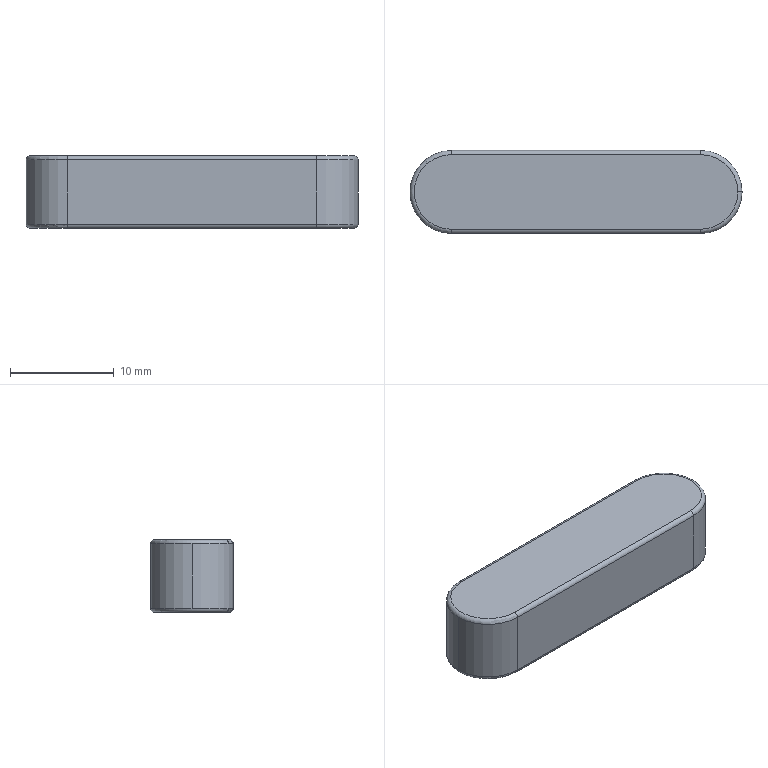Part | SolidWorks | features BaseBody 1 | 1 solid | 17 faces | box 32 x 8 x 7 mm | volume 1691 mm3 | cylinder 7 | torus 6 | plane 4 | commonest cylinder face diameters 0.8 x4 8 x3
STEP:
#1=CARTESIAN_POINT('',(15.6,0.,0.));
#2=VERTEX_POINT('',#1);
#3=CARTESIAN_POINT('',(16.,0.,0.4));
#4=VERTEX_POINT('',#3);
#5=CARTESIAN_POINT('',(15.6,0.,0.4));
#6=DIRECTION('',(0.,-1.,0.));
#7=DIRECTION('',(1.,0.,0.));
#8=AXIS2_PLACEMENT_3D('',#5,#6,#7);
#9=CIRCLE('',#8,0.4);
#10=EDGE_CURVE('',#2,#4,#9,.T.);
#11=ORIENTED_EDGE('',*,*,#10,.F.);
#12=CARTESIAN_POINT('',(12.,3.6,0.));
#13=VERTEX_POINT('',#12);
#14=CARTESIAN_POINT('',(12.,0.,0.));
#15=DIRECTION('',(0.,0.,-1.));
#16=DIRECTION('',(1.,0.,0.));
#17=AXIS2_PLACEMENT_3D('',#14,#15,#16);
#18=CIRCLE('',#17,3.6);
#19=EDGE_CURVE('',#13,#2,#18,.T.);
#20=ORIENTED_EDGE('',*,*,#19,.F.);
#21=CARTESIAN_POINT('',(12.,4.,0.4));
#22=VERTEX_POINT('',#21);
#23=CARTESIAN_POINT('',(12.,3.6,0.4));
#24=DIRECTION('',(1.,0.,0.));
#25=DIRECTION('',(0.,0.,-1.));
#26=AXIS2_PLACEMENT_3D('',#23,#24,#25);
#27=CIRCLE('',#26,0.4);
#28=EDGE_CURVE('',#13,#22,#27,.T.);
#29=ORIENTED_EDGE('',*,*,#28,.T.);
#30=CARTESIAN_POINT('',(12.,0.,0.4));
#31=DIRECTION('',(0.,0.,1.));
#32=DIRECTION('',(1.,0.,0.));
#33=AXIS2_PLACEMENT_3D('',#30,#31,#32);
#34=CIRCLE('',#33,4.);
#35=EDGE_CURVE('',#4,#22,#34,.T.);
#36=ORIENTED_EDGE('',*,*,#35,.F.);
#37=EDGE_LOOP('',(#11,#20,#29,#36));
#38=FACE_OUTER_BOUND('',#37,.T.);
#39=CARTESIAN_POINT('',(12.,0.,0.4));
#40=DIRECTION('',(0.,0.,1.));
#41=DIRECTION('',(1.,0.,0.));
#42=AXIS2_PLACEMENT_3D('',#39,#40,#41);
#43=TOROIDAL_SURFACE('',#42,3.6,0.4);
#44=ADVANCED_FACE('',(#38),#43,.T.);
#45=CARTESIAN_POINT('',(-12.,3.6,0.));
#46=VERTEX_POINT('',#45);
#47=CARTESIAN_POINT('',(-12.,4.,0.4));
#48=VERTEX_POINT('',#47);
#49=CARTESIAN_POINT('',(-12.,3.6,0.4));
#50=DIRECTION('',(1.,0.,0.));
#51=DIRECTION('',(0.,0.,-1.));
#52=AXIS2_PLACEMENT_3D('',#49,#50,#51);
#53=CIRCLE('',#52,0.4);
#54=EDGE_CURVE('',#46,#48,#53,.T.);
#55=ORIENTED_EDGE('',*,*,#54,.T.);
#56=CARTESIAN_POINT('',(-12.,4.,0.4));
#57=DIRECTION('',(-1.,0.,0.));
#58=VECTOR('',#57,1000.);
#59=LINE('',#56,#58);
#60=EDGE_CURVE('',#22,#48,#59,.T.);
#61=ORIENTED_EDGE('',*,*,#60,.F.);
#62=ORIENTED_EDGE('',*,*,#28,.F.);
#63=CARTESIAN_POINT('',(-12.,3.6,0.));
#64=DIRECTION('',(1.,0.,0.));
#65=VECTOR('',#64,1000.);
#66=LINE('',#63,#65);
#67=EDGE_CURVE('',#46,#13,#66,.T.);
#68=ORIENTED_EDGE('',*,*,#67,.F.);
#69=EDGE_LOOP('',(#55,#61,#62,#68));
#70=FACE_OUTER_BOUND('',#69,.T.);
#71=CARTESIAN_POINT('',(-12.,3.6,0.4));
#72=DIRECTION('',(-1.,0.,0.));
#73=DIRECTION('',(0.,-1.,0.));
#74=AXIS2_PLACEMENT_3D('',#71,#72,#73);
#75=CYLINDRICAL_SURFACE('',#74,0.4);
#76=ADVANCED_FACE('',(#70),#75,.T.);
#77=CARTESIAN_POINT('',(-12.,-4.,0.4));
#78=VERTEX_POINT('',#77);
#79=CARTESIAN_POINT('',(-12.,-3.6,0.));
#80=VERTEX_POINT('',#79);
#81=CARTESIAN_POINT('',(-12.,-3.6,0.4));
#82=DIRECTION('',(1.,0.,0.));
#83=DIRECTION('',(0.,0.,-1.));
#84=AXIS2_PLACEMENT_3D('',#81,#82,#83);
#85=CIRCLE('',#84,0.4);
#86=EDGE_CURVE('',#78,#80,#85,.T.);
#87=ORIENTED_EDGE('',*,*,#86,.T.);
#88=CARTESIAN_POINT('',(12.,-3.6,0.));
#89=VERTEX_POINT('',#88);
#90=CARTESIAN_POINT('',(-12.,-3.6,0.));
#91=DIRECTION('',(-1.,0.,0.));
#92=VECTOR('',#91,1000.);
#93=LINE('',#90,#92);
#94=EDGE_CURVE('',#89,#80,#93,.T.);
#95=ORIENTED_EDGE('',*,*,#94,.F.);
#96=CARTESIAN_POINT('',(12.,-4.,0.4));
#97=VERTEX_POINT('',#96);
#98=CARTESIAN_POINT('',(12.,-3.6,0.4));
#99=DIRECTION('',(1.,0.,0.));
#100=DIRECTION('',(0.,0.,-1.));
#101=AXIS2_PLACEMENT_3D('',#98,#99,#100);
#102=CIRCLE('',#101,0.4);
#103=EDGE_CURVE('',#97,#89,#102,.T.);
#104=ORIENTED_EDGE('',*,*,#103,.F.);
#105=CARTESIAN_POINT('',(-12.,-4.,0.4));
#106=DIRECTION('',(1.,0.,0.));
#107=VECTOR('',#106,1000.);
#108=LINE('',#105,#107);
#109=EDGE_CURVE('',#78,#97,#108,.T.);
#110=ORIENTED_EDGE('',*,*,#109,.F.);
#111=EDGE_LOOP('',(#87,#95,#104,#110));
#112=FACE_OUTER_BOUND('',#111,.T.);
#113=CARTESIAN_POINT('',(-12.,-3.6,0.4));
#114=DIRECTION('',(1.,0.,0.));
#115=DIRECTION('',(0.,1.,0.));
#116=AXIS2_PLACEMENT_3D('',#113,#114,#115);
#117=CYLINDRICAL_SURFACE('',#116,0.4);
#118=ADVANCED_FACE('',(#112),#117,.T.);
#119=ORIENTED_EDGE('',*,*,#54,.F.);
#120=CARTESIAN_POINT('',(-12.,0.,0.));
#121=DIRECTION('',(0.,0.,-1.));
#122=DIRECTION('',(1.,0.,0.));
#123=AXIS2_PLACEMENT_3D('',#120,#121,#122);
#124=CIRCLE('',#123,3.6);
#125=EDGE_CURVE('',#80,#46,#124,.T.);
#126=ORIENTED_EDGE('',*,*,#125,.F.);
#127=ORIENTED_EDGE('',*,*,#86,.F.);
#128=CARTESIAN_POINT('',(-16.,0.,0.4));
#129=VERTEX_POINT('',#128);
#130=CARTESIAN_POINT('',(-12.,0.,0.4));
#131=DIRECTION('',(0.,0.,1.));
#132=DIRECTION('',(1.,0.,0.));
#133=AXIS2_PLACEMENT_3D('',#130,#131,#132);
#134=CIRCLE('',#133,4.);
#135=EDGE_CURVE('',#129,#78,#134,.T.);
#136=ORIENTED_EDGE('',*,*,#135,.F.);
#137=CARTESIAN_POINT('',(-12.,0.,0.4));
#138=DIRECTION('',(0.,0.,1.));
#139=DIRECTION('',(1.,0.,0.));
#140=AXIS2_PLACEMENT_3D('',#137,#138,#139);
#141=CIRCLE('',#140,4.);
#142=EDGE_CURVE('',#48,#129,#141,.T.);
#143=ORIENTED_EDGE('',*,*,#142,.F.);
#144=EDGE_LOOP('',(#119,#126,#127,#136,#143));
#145=FACE_OUTER_BOUND('',#144,.T.);
#146=CARTESIAN_POINT('',(-12.,0.,0.4));
#147=DIRECTION('',(0.,0.,1.));
#148=DIRECTION('',(1.,0.,0.));
#149=AXIS2_PLACEMENT_3D('',#146,#147,#148);
#150=TOROIDAL_SURFACE('',#149,3.6,0.4);
#151=ADVANCED_FACE('',(#145),#150,.T.);
#152=CARTESIAN_POINT('',(16.,0.,6.6));
#153=VERTEX_POINT('',#152);
#154=CARTESIAN_POINT('',(15.6,0.,7.));
#155=VERTEX_POINT('',#154);
#156=CARTESIAN_POINT('',(15.6,0.,6.6));
#157=DIRECTION('',(0.,-1.,0.));
#158=DIRECTION('',(1.,0.,0.));
#159=AXIS2_PLACEMENT_3D('',#156,#157,#158);
#160=CIRCLE('',#159,0.4);
#161=EDGE_CURVE('',#153,#155,#160,.T.);
#162=ORIENTED_EDGE('',*,*,#161,.F.);
#163=CARTESIAN_POINT('',(12.,4.,6.6));
#164=VERTEX_POINT('',#163);
#165=CARTESIAN_POINT('',(12.,0.,6.6));
#166=DIRECTION('',(0.,0.,-1.));
#167=DIRECTION('',(1.,0.,0.));
#168=AXIS2_PLACEMENT_3D('',#165,#166,#167);
#169=CIRCLE('',#168,4.);
#170=EDGE_CURVE('',#164,#153,#169,.T.);
#171=ORIENTED_EDGE('',*,*,#170,.F.);
#172=CARTESIAN_POINT('',(12.,3.6,7.));
#173=VERTEX_POINT('',#172);
#174=CARTESIAN_POINT('',(12.,3.6,6.6));
#175=DIRECTION('',(1.,0.,0.));
#176=DIRECTION('',(0.,0.,-1.));
#177=AXIS2_PLACEMENT_3D('',#174,#175,#176);
#178=CIRCLE('',#177,0.4);
#179=EDGE_CURVE('',#164,#173,#178,.T.);
#180=ORIENTED_EDGE('',*,*,#179,.T.);
#181=CARTESIAN_POINT('',(12.,0.,7.));
#182=DIRECTION('',(0.,0.,1.));
#183=DIRECTION('',(1.,0.,0.));
#184=AXIS2_PLACEMENT_3D('',#181,#182,#183);
#185=CIRCLE('',#184,3.6);
#186=EDGE_CURVE('',#155,#173,#185,.T.);
#187=ORIENTED_EDGE('',*,*,#186,.F.);
#188=EDGE_LOOP('',(#162,#171,#180,#187));
#189=FACE_OUTER_BOUND('',#188,.T.);
#190=CARTESIAN_POINT('',(12.,0.,6.6));
#191=DIRECTION('',(0.,0.,1.));
#192=DIRECTION('',(1.,0.,0.));
#193=AXIS2_PLACEMENT_3D('',#190,#191,#192);
#194=TOROIDAL_SURFACE('',#193,3.6,0.4);
#195=ADVANCED_FACE('',(#189),#194,.T.);
#196=CARTESIAN_POINT('',(-12.,4.,6.6));
#197=VERTEX_POINT('',#196);
#198=CARTESIAN_POINT('',(-12.,3.6,7.));
#199=VERTEX_POINT('',#198);
#200=CARTESIAN_POINT('',(-12.,3.6,6.6));
#201=DIRECTION('',(1.,0.,0.));
#202=DIRECTION('',(0.,0.,-1.));
#203=AXIS2_PLACEMENT_3D('',#200,#201,#202);
#204=CIRCLE('',#203,0.4);
#205=EDGE_CURVE('',#197,#199,#204,.T.);
#206=ORIENTED_EDGE('',*,*,#205,.T.);
#207=CARTESIAN_POINT('',(-12.,3.6,7.));
#208=DIRECTION('',(-1.,0.,0.));
#209=VECTOR('',#208,1000.);
#210=LINE('',#207,#209);
#211=EDGE_CURVE('',#173,#199,#210,.T.);
#212=ORIENTED_EDGE('',*,*,#211,.F.);
#213=ORIENTED_EDGE('',*,*,#179,.F.);
#214=CARTESIAN_POINT('',(12.,4.,6.6));
#215=DIRECTION('',(1.,0.,0.));
#216=VECTOR('',#215,1000.);
#217=LINE('',#214,#216);
#218=EDGE_CURVE('',#197,#164,#217,.T.);
#219=ORIENTED_EDGE('',*,*,#218,.F.);
#220=EDGE_LOOP('',(#206,#212,#213,#219));
#221=FACE_OUTER_BOUND('',#220,.T.);
#222=CARTESIAN_POINT('',(-12.,3.6,6.6));
#223=DIRECTION('',(1.,0.,0.));
#224=DIRECTION('',(0.,1.,0.));
#225=AXIS2_PLACEMENT_3D('',#222,#223,#224);
#226=CYLINDRICAL_SURFACE('',#225,0.4);
#227=ADVANCED_FACE('',(#221),#226,.T.);
#228=CARTESIAN_POINT('',(-12.,-3.6,7.));
#229=VERTEX_POINT('',#228);
#230=CARTESIAN_POINT('',(-12.,-4.,6.6));
#231=VERTEX_POINT('',#230);
#232=CARTESIAN_POINT('',(-12.,-3.6,6.6));
#233=DIRECTION('',(1.,0.,0.));
#234=DIRECTION('',(0.,0.,-1.));
#235=AXIS2_PLACEMENT_3D('',#232,#233,#234);
#236=CIRCLE('',#235,0.4);
#237=EDGE_CURVE('',#229,#231,#236,.T.);
#238=ORIENTED_EDGE('',*,*,#237,.T.);
#239=CARTESIAN_POINT('',(12.,-4.,6.6));
#240=VERTEX_POINT('',#239);
#241=CARTESIAN_POINT('',(-12.,-4.,6.6));
#242=DIRECTION('',(-1.,0.,0.));
#243=VECTOR('',#242,1000.);
#244=LINE('',#241,#243);
#245=EDGE_CURVE('',#240,#231,#244,.T.);
#246=ORIENTED_EDGE('',*,*,#245,.F.);
#247=CARTESIAN_POINT('',(12.,-3.6,7.));
#248=VERTEX_POINT('',#247);
#249=CARTESIAN_POINT('',(12.,-3.6,6.6));
#250=DIRECTION('',(1.,0.,0.));
#251=DIRECTION('',(0.,0.,-1.));
#252=AXIS2_PLACEMENT_3D('',#249,#250,#251);
#253=CIRCLE('',#252,0.4);
#254=EDGE_CURVE('',#248,#240,#253,.T.);
#255=ORIENTED_EDGE('',*,*,#254,.F.);
#256=CARTESIAN_POINT('',(12.,-3.6,7.));
#257=DIRECTION('',(1.,0.,0.));
#258=VECTOR('',#257,1000.);
#259=LINE('',#256,#258);
#260=EDGE_CURVE('',#229,#248,#259,.T.);
#261=ORIENTED_EDGE('',*,*,#260,.F.);
#262=EDGE_LOOP('',(#238,#246,#255,#261));
#263=FACE_OUTER_BOUND('',#262,.T.);
#264=CARTESIAN_POINT('',(-12.,-3.6,6.6));
#265=DIRECTION('',(-1.,0.,0.));
#266=DIRECTION('',(0.,-1.,0.));
#267=AXIS2_PLACEMENT_3D('',#264,#265,#266);
#268=CYLINDRICAL_SURFACE('',#267,0.4);
#269=ADVANCED_FACE('',(#263),#268,.T.);
#270=ORIENTED_EDGE('',*,*,#205,.F.);
#271=CARTESIAN_POINT('',(-16.,0.,6.6));
#272=VERTEX_POINT('',#271);
#273=CARTESIAN_POINT('',(-12.,0.,6.6));
#274=DIRECTION('',(0.,0.,-1.));
#275=DIRECTION('',(1.,0.,0.));
#276=AXIS2_PLACEMENT_3D('',#273,#274,#275);
#277=CIRCLE('',#276,4.);
#278=EDGE_CURVE('',#272,#197,#277,.T.);
#279=ORIENTED_EDGE('',*,*,#278,.F.);
#280=CARTESIAN_POINT('',(-12.,0.,6.6));
#281=DIRECTION('',(0.,0.,-1.));
#282=DIRECTION('',(1.,0.,0.));
#283=AXIS2_PLACEMENT_3D('',#280,#281,#282);
#284=CIRCLE('',#283,4.);
#285=EDGE_CURVE('',#231,#272,#284,.T.);
#286=ORIENTED_EDGE('',*,*,#285,.F.);
#287=ORIENTED_EDGE('',*,*,#237,.F.);
#288=CARTESIAN_POINT('',(-12.,0.,7.));
#289=DIRECTION('',(0.,0.,1.));
#290=DIRECTION('',(1.,0.,0.));
#291=AXIS2_PLACEMENT_3D('',#288,#289,#290);
#292=CIRCLE('',#291,3.6);
#293=EDGE_CURVE('',#199,#229,#292,.T.);
#294=ORIENTED_EDGE('',*,*,#293,.F.);
#295=EDGE_LOOP('',(#270,#279,#286,#287,#294));
#296=FACE_OUTER_BOUND('',#295,.T.);
#297=CARTESIAN_POINT('',(-12.,0.,6.6));
#298=DIRECTION('',(0.,0.,1.));
#299=DIRECTION('',(1.,0.,0.));
#300=AXIS2_PLACEMENT_3D('',#297,#298,#299);
#301=TOROIDAL_SURFACE('',#300,3.6,0.4);
#302=ADVANCED_FACE('',(#296),#301,.T.);
#303=ORIENTED_EDGE('',*,*,#67,.T.);
#304=ORIENTED_EDGE('',*,*,#19,.T.);
#305=CARTESIAN_POINT('',(12.,0.,0.));
#306=DIRECTION('',(0.,0.,-1.));
#307=DIRECTION('',(1.,0.,0.));
#308=AXIS2_PLACEMENT_3D('',#305,#306,#307);
#309=CIRCLE('',#308,3.6);
#310=EDGE_CURVE('',#2,#89,#309,.T.);
#311=ORIENTED_EDGE('',*,*,#310,.T.);
#312=ORIENTED_EDGE('',*,*,#94,.T.);
#313=ORIENTED_EDGE('',*,*,#125,.T.);
#314=EDGE_LOOP('',(#303,#304,#311,#312,#313));
#315=FACE_OUTER_BOUND('',#314,.T.);
#316=CARTESIAN_POINT('',(-12.,0.,0.));
#317=DIRECTION('',(0.,0.,1.));
#318=DIRECTION('',(0.,-1.,0.));
#319=AXIS2_PLACEMENT_3D('',#316,#317,#318);
#320=PLANE('',#319);
#321=ADVANCED_FACE('',(#315),#320,.F.);
#322=ORIENTED_EDGE('',*,*,#260,.T.);
#323=CARTESIAN_POINT('',(12.,0.,7.));
#324=DIRECTION('',(0.,0.,1.));
#325=DIRECTION('',(1.,0.,0.));
#326=AXIS2_PLACEMENT_3D('',#323,#324,#325);
#327=CIRCLE('',#326,3.6);
#328=EDGE_CURVE('',#248,#155,#327,.T.);
#329=ORIENTED_EDGE('',*,*,#328,.T.);
#330=ORIENTED_EDGE('',*,*,#186,.T.);
#331=ORIENTED_EDGE('',*,*,#211,.T.);
#332=ORIENTED_EDGE('',*,*,#293,.T.);
#333=EDGE_LOOP('',(#322,#329,#330,#331,#332));
#334=FACE_OUTER_BOUND('',#333,.T.);
#335=CARTESIAN_POINT('',(-12.,0.,7.));
#336=DIRECTION('',(0.,0.,1.));
#337=DIRECTION('',(0.,-1.,0.));
#338=AXIS2_PLACEMENT_3D('',#335,#336,#337);
#339=PLANE('',#338);
#340=ADVANCED_FACE('',(#334),#339,.T.);
#341=CARTESIAN_POINT('',(-12.,4.,7.));
#342=DIRECTION('',(0.,0.,-1.));
#343=VECTOR('',#342,1000.);
#344=LINE('',#341,#343);
#345=EDGE_CURVE('',#197,#48,#344,.T.);
#346=ORIENTED_EDGE('',*,*,#345,.F.);
#347=ORIENTED_EDGE('',*,*,#218,.T.);
#348=CARTESIAN_POINT('',(12.,4.,7.));
#349=DIRECTION('',(0.,0.,-1.));
#350=VECTOR('',#349,1000.);
#351=LINE('',#348,#350);
#352=EDGE_CURVE('',#164,#22,#351,.T.);
#353=ORIENTED_EDGE('',*,*,#352,.T.);
#354=ORIENTED_EDGE('',*,*,#60,.T.);
#355=EDGE_LOOP('',(#346,#347,#353,#354));
#356=FACE_OUTER_BOUND('',#355,.T.);
#357=CARTESIAN_POINT('',(-12.,4.,7.));
#358=DIRECTION('',(0.,-1.,0.));
#359=DIRECTION('',(0.,0.,-1.));
#360=AXIS2_PLACEMENT_3D('',#357,#358,#359);
#361=PLANE('',#360);
#362=ADVANCED_FACE('',(#356),#361,.F.);
#363=ORIENTED_EDGE('',*,*,#352,.F.);
#364=ORIENTED_EDGE('',*,*,#170,.T.);
#365=CARTESIAN_POINT('',(12.,0.,6.6));
#366=DIRECTION('',(0.,0.,-1.));
#367=DIRECTION('',(1.,0.,0.));
#368=AXIS2_PLACEMENT_3D('',#365,#366,#367);
#369=CIRCLE('',#368,4.);
#370=EDGE_CURVE('',#153,#240,#369,.T.);
#371=ORIENTED_EDGE('',*,*,#370,.T.);
#372=CARTESIAN_POINT('',(12.,-4.,7.));
#373=DIRECTION('',(0.,0.,-1.));
#374=VECTOR('',#373,1000.);
#375=LINE('',#372,#374);
#376=EDGE_CURVE('',#240,#97,#375,.T.);
#377=ORIENTED_EDGE('',*,*,#376,.T.);
#378=CARTESIAN_POINT('',(12.,0.,0.4));
#379=DIRECTION('',(0.,0.,1.));
#380=DIRECTION('',(1.,0.,0.));
#381=AXIS2_PLACEMENT_3D('',#378,#379,#380);
#382=CIRCLE('',#381,4.);
#383=EDGE_CURVE('',#97,#4,#382,.T.);
#384=ORIENTED_EDGE('',*,*,#383,.T.);
#385=ORIENTED_EDGE('',*,*,#35,.T.);
#386=EDGE_LOOP('',(#363,#364,#371,#377,#384,#385));
#387=FACE_OUTER_BOUND('',#386,.T.);
#388=CARTESIAN_POINT('',(12.,0.,7.));
#389=DIRECTION('',(0.,0.,-1.));
#390=DIRECTION('',(-1.,0.,0.));
#391=AXIS2_PLACEMENT_3D('',#388,#389,#390);
#392=CYLINDRICAL_SURFACE('',#391,4.);
#393=ADVANCED_FACE('',(#387),#392,.T.);
#394=ORIENTED_EDGE('',*,*,#376,.F.);
#395=ORIENTED_EDGE('',*,*,#245,.T.);
#396=CARTESIAN_POINT('',(-12.,-4.,7.));
#397=DIRECTION('',(0.,0.,-1.));
#398=VECTOR('',#397,1000.);
#399=LINE('',#396,#398);
#400=EDGE_CURVE('',#231,#78,#399,.T.);
#401=ORIENTED_EDGE('',*,*,#400,.T.);
#402=ORIENTED_EDGE('',*,*,#109,.T.);
#403=EDGE_LOOP('',(#394,#395,#401,#402));
#404=FACE_OUTER_BOUND('',#403,.T.);
#405=CARTESIAN_POINT('',(-12.,-4.,7.));
#406=DIRECTION('',(0.,1.,0.));
#407=DIRECTION('',(1.,0.,0.));
#408=AXIS2_PLACEMENT_3D('',#405,#406,#407);
#409=PLANE('',#408);
#410=ADVANCED_FACE('',(#404),#409,.F.);
#411=CARTESIAN_POINT('',(-16.,0.,7.));
#412=DIRECTION('',(0.,0.,-1.));
#413=VECTOR('',#412,1000.);
#414=LINE('',#411,#413);
#415=EDGE_CURVE('',#272,#129,#414,.T.);
#416=ORIENTED_EDGE('',*,*,#415,.F.);
#417=ORIENTED_EDGE('',*,*,#278,.T.);
#418=ORIENTED_EDGE('',*,*,#345,.T.);
#419=ORIENTED_EDGE('',*,*,#142,.T.);
#420=EDGE_LOOP('',(#416,#417,#418,#419));
#421=FACE_OUTER_BOUND('',#420,.T.);
#422=CARTESIAN_POINT('',(-12.,0.,7.));
#423=DIRECTION('',(0.,0.,-1.));
#424=DIRECTION('',(-1.,0.,0.));
#425=AXIS2_PLACEMENT_3D('',#422,#423,#424);
#426=CYLINDRICAL_SURFACE('',#425,4.);
#427=ADVANCED_FACE('',(#421),#426,.T.);
#428=ORIENTED_EDGE('',*,*,#285,.T.);
#429=ORIENTED_EDGE('',*,*,#415,.T.);
#430=ORIENTED_EDGE('',*,*,#135,.T.);
#431=ORIENTED_EDGE('',*,*,#400,.F.);
#432=EDGE_LOOP('',(#428,#429,#430,#431));
#433=FACE_OUTER_BOUND('',#432,.T.);
#434=CARTESIAN_POINT('',(-12.,0.,7.));
#435=DIRECTION('',(0.,0.,-1.));
#436=DIRECTION('',(-1.,0.,0.));
#437=AXIS2_PLACEMENT_3D('',#434,#435,#436);
#438=CYLINDRICAL_SURFACE('',#437,4.);
#439=ADVANCED_FACE('',(#433),#438,.T.);
#440=ORIENTED_EDGE('',*,*,#370,.F.);
#441=ORIENTED_EDGE('',*,*,#161,.T.);
#442=ORIENTED_EDGE('',*,*,#328,.F.);
#443=ORIENTED_EDGE('',*,*,#254,.T.);
#444=EDGE_LOOP('',(#440,#441,#442,#443));
#445=FACE_OUTER_BOUND('',#444,.T.);
#446=CARTESIAN_POINT('',(12.,0.,6.6));
#447=DIRECTION('',(0.,0.,1.));
#448=DIRECTION('',(1.,0.,0.));
#449=AXIS2_PLACEMENT_3D('',#446,#447,#448);
#450=TOROIDAL_SURFACE('',#449,3.6,0.4);
#451=ADVANCED_FACE('',(#445),#450,.T.);
#452=ORIENTED_EDGE('',*,*,#310,.F.);
#453=ORIENTED_EDGE('',*,*,#10,.T.);
#454=ORIENTED_EDGE('',*,*,#383,.F.);
#455=ORIENTED_EDGE('',*,*,#103,.T.);
#456=EDGE_LOOP('',(#452,#453,#454,#455));
#457=FACE_OUTER_BOUND('',#456,.T.);
#458=CARTESIAN_POINT('',(12.,0.,0.4));
#459=DIRECTION('',(0.,0.,1.));
#460=DIRECTION('',(1.,0.,0.));
#461=AXIS2_PLACEMENT_3D('',#458,#459,#460);
#462=TOROIDAL_SURFACE('',#461,3.6,0.4);
#463=ADVANCED_FACE('',(#457),#462,.T.);
#464=CLOSED_SHELL('',(#44,#76,#118,#151,#195,#227,#269,#302,#321,#340,#362,#393,#410,#427,#439,#451,#463));
#465=MANIFOLD_SOLID_BREP('',#464);
#466=CARTESIAN_POINT('',(0.,0.,0.));
#467=DIRECTION('',(0.,0.,1.));
#468=DIRECTION('',(1.,0.,0.));
#469=AXIS2_PLACEMENT_3D('',#466,#467,#468);
#470=(LENGTH_UNIT()NAMED_UNIT(*)SI_UNIT(.MILLI.,.METRE.));
#471=UNCERTAINTY_MEASURE_WITH_UNIT(LENGTH_MEASURE(0.00001),#470,'','');
#472=(NAMED_UNIT(*)PLANE_ANGLE_UNIT()SI_UNIT($,.RADIAN.));
#473=(NAMED_UNIT(*)SI_UNIT($,.STERADIAN.)SOLID_ANGLE_UNIT());
#474=(GEOMETRIC_REPRESENTATION_CONTEXT(3)GLOBAL_UNCERTAINTY_ASSIGNED_CONTEXT((#471))GLOBAL_UNIT_ASSIGNED_CONTEXT((#470,#472,#473))REPRESENTATION_CONTEXT('',''));
#475=ADVANCED_BREP_SHAPE_REPRESENTATION('',(#465,#469),#474);